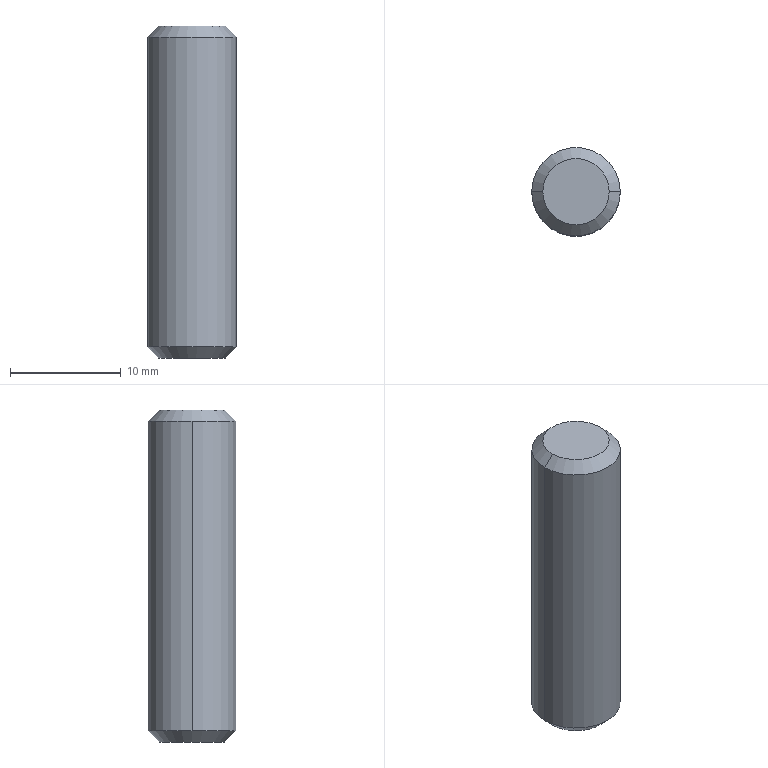Part | SolidWorks | features Chamfer 1, Extrusion 1 | 1 solid | 8 faces | box 8 x 8 x 30 mm | volume 1485 mm3 | cone 4 | cylinder 2 | plane 2 | commonest cylinder face diameters 8 x2
STEP:
#1=CARTESIAN_POINT('',(3.,0.,30.));
#2=VERTEX_POINT('',#1);
#3=CARTESIAN_POINT('',(-3.,0.,30.));
#4=VERTEX_POINT('',#3);
#5=CARTESIAN_POINT('',(0.,0.,30.));
#6=DIRECTION('',(0.,0.,1.));
#7=DIRECTION('',(1.,0.,0.));
#8=AXIS2_PLACEMENT_3D('',#5,#6,#7);
#9=CIRCLE('',#8,3.);
#10=EDGE_CURVE('',#2,#4,#9,.T.);
#11=ORIENTED_EDGE('',*,*,#10,.F.);
#12=CARTESIAN_POINT('',(4.,0.,29.));
#13=VERTEX_POINT('',#12);
#14=CARTESIAN_POINT('',(3.,0.,30.));
#15=DIRECTION('',(0.7071,0.,-0.7071));
#16=VECTOR('',#15,1000.);
#17=LINE('',#14,#16);
#18=EDGE_CURVE('',#2,#13,#17,.T.);
#19=ORIENTED_EDGE('',*,*,#18,.T.);
#20=CARTESIAN_POINT('',(-4.,0.,29.));
#21=VERTEX_POINT('',#20);
#22=CARTESIAN_POINT('',(0.,0.,29.));
#23=DIRECTION('',(0.,0.,-1.));
#24=DIRECTION('',(1.,0.,0.));
#25=AXIS2_PLACEMENT_3D('',#22,#23,#24);
#26=CIRCLE('',#25,4.);
#27=EDGE_CURVE('',#21,#13,#26,.T.);
#28=ORIENTED_EDGE('',*,*,#27,.F.);
#29=CARTESIAN_POINT('',(-3.,0.,30.));
#30=DIRECTION('',(-0.7071,0.,-0.7071));
#31=VECTOR('',#30,1000.);
#32=LINE('',#29,#31);
#33=EDGE_CURVE('',#4,#21,#32,.T.);
#34=ORIENTED_EDGE('',*,*,#33,.F.);
#35=EDGE_LOOP('',(#11,#19,#28,#34));
#36=FACE_OUTER_BOUND('',#35,.T.);
#37=CARTESIAN_POINT('',(0.,0.,30.));
#38=DIRECTION('',(0.,0.,-1.));
#39=DIRECTION('',(-1.,0.,0.));
#40=AXIS2_PLACEMENT_3D('',#37,#38,#39);
#41=CONICAL_SURFACE('',#40,3.,0.7854);
#42=ADVANCED_FACE('',(#36),#41,.T.);
#43=CARTESIAN_POINT('',(-3.,0.,0.));
#44=VERTEX_POINT('',#43);
#45=CARTESIAN_POINT('',(3.,0.,0.));
#46=VERTEX_POINT('',#45);
#47=CARTESIAN_POINT('',(0.,0.,0.));
#48=DIRECTION('',(0.,0.,-1.));
#49=DIRECTION('',(1.,0.,0.));
#50=AXIS2_PLACEMENT_3D('',#47,#48,#49);
#51=CIRCLE('',#50,3.);
#52=EDGE_CURVE('',#44,#46,#51,.T.);
#53=ORIENTED_EDGE('',*,*,#52,.F.);
#54=CARTESIAN_POINT('',(-4.,0.,1.));
#55=VERTEX_POINT('',#54);
#56=CARTESIAN_POINT('',(-4.,0.,1.));
#57=DIRECTION('',(-0.7071,0.,0.7071));
#58=VECTOR('',#57,1000.);
#59=LINE('',#56,#58);
#60=EDGE_CURVE('',#44,#55,#59,.T.);
#61=ORIENTED_EDGE('',*,*,#60,.T.);
#62=CARTESIAN_POINT('',(4.,0.,1.));
#63=VERTEX_POINT('',#62);
#64=CARTESIAN_POINT('',(0.,0.,1.));
#65=DIRECTION('',(0.,0.,1.));
#66=DIRECTION('',(1.,0.,0.));
#67=AXIS2_PLACEMENT_3D('',#64,#65,#66);
#68=CIRCLE('',#67,4.);
#69=EDGE_CURVE('',#63,#55,#68,.T.);
#70=ORIENTED_EDGE('',*,*,#69,.F.);
#71=CARTESIAN_POINT('',(4.,0.,1.));
#72=DIRECTION('',(0.7071,0.,0.7071));
#73=VECTOR('',#72,1000.);
#74=LINE('',#71,#73);
#75=EDGE_CURVE('',#46,#63,#74,.T.);
#76=ORIENTED_EDGE('',*,*,#75,.F.);
#77=EDGE_LOOP('',(#53,#61,#70,#76));
#78=FACE_OUTER_BOUND('',#77,.T.);
#79=CARTESIAN_POINT('',(0.,0.,1.));
#80=DIRECTION('',(0.,0.,1.));
#81=DIRECTION('',(1.,0.,0.));
#82=AXIS2_PLACEMENT_3D('',#79,#80,#81);
#83=CONICAL_SURFACE('',#82,4.,0.7854);
#84=ADVANCED_FACE('',(#78),#83,.T.);
#85=ORIENTED_EDGE('',*,*,#27,.T.);
#86=CARTESIAN_POINT('',(4.,0.,30.));
#87=DIRECTION('',(0.,0.,-1.));
#88=VECTOR('',#87,1000.);
#89=LINE('',#86,#88);
#90=EDGE_CURVE('',#13,#63,#89,.T.);
#91=ORIENTED_EDGE('',*,*,#90,.T.);
#92=ORIENTED_EDGE('',*,*,#69,.T.);
#93=CARTESIAN_POINT('',(-4.,0.,30.));
#94=DIRECTION('',(0.,0.,-1.));
#95=VECTOR('',#94,1000.);
#96=LINE('',#93,#95);
#97=EDGE_CURVE('',#21,#55,#96,.T.);
#98=ORIENTED_EDGE('',*,*,#97,.F.);
#99=EDGE_LOOP('',(#85,#91,#92,#98));
#100=FACE_OUTER_BOUND('',#99,.T.);
#101=CARTESIAN_POINT('',(0.,0.,30.));
#102=DIRECTION('',(0.,0.,-1.));
#103=DIRECTION('',(-1.,0.,0.));
#104=AXIS2_PLACEMENT_3D('',#101,#102,#103);
#105=CYLINDRICAL_SURFACE('',#104,4.);
#106=ADVANCED_FACE('',(#100),#105,.T.);
#107=ORIENTED_EDGE('',*,*,#90,.F.);
#108=CARTESIAN_POINT('',(0.,0.,29.));
#109=DIRECTION('',(0.,0.,-1.));
#110=DIRECTION('',(1.,0.,0.));
#111=AXIS2_PLACEMENT_3D('',#108,#109,#110);
#112=CIRCLE('',#111,4.);
#113=EDGE_CURVE('',#13,#21,#112,.T.);
#114=ORIENTED_EDGE('',*,*,#113,.T.);
#115=ORIENTED_EDGE('',*,*,#97,.T.);
#116=CARTESIAN_POINT('',(0.,0.,1.));
#117=DIRECTION('',(0.,0.,1.));
#118=DIRECTION('',(1.,0.,0.));
#119=AXIS2_PLACEMENT_3D('',#116,#117,#118);
#120=CIRCLE('',#119,4.);
#121=EDGE_CURVE('',#55,#63,#120,.T.);
#122=ORIENTED_EDGE('',*,*,#121,.T.);
#123=EDGE_LOOP('',(#107,#114,#115,#122));
#124=FACE_OUTER_BOUND('',#123,.T.);
#125=CARTESIAN_POINT('',(0.,0.,30.));
#126=DIRECTION('',(0.,0.,-1.));
#127=DIRECTION('',(-1.,0.,0.));
#128=AXIS2_PLACEMENT_3D('',#125,#126,#127);
#129=CYLINDRICAL_SURFACE('',#128,4.);
#130=ADVANCED_FACE('',(#124),#129,.T.);
#131=CARTESIAN_POINT('',(0.,0.,30.));
#132=DIRECTION('',(0.,0.,1.));
#133=DIRECTION('',(1.,0.,0.));
#134=AXIS2_PLACEMENT_3D('',#131,#132,#133);
#135=CIRCLE('',#134,3.);
#136=EDGE_CURVE('',#4,#2,#135,.T.);
#137=ORIENTED_EDGE('',*,*,#136,.T.);
#138=ORIENTED_EDGE('',*,*,#10,.T.);
#139=EDGE_LOOP('',(#137,#138));
#140=FACE_OUTER_BOUND('',#139,.T.);
#141=CARTESIAN_POINT('',(0.,0.,30.));
#142=DIRECTION('',(0.,0.,1.));
#143=DIRECTION('',(1.,0.,0.));
#144=AXIS2_PLACEMENT_3D('',#141,#142,#143);
#145=PLANE('',#144);
#146=ADVANCED_FACE('',(#140),#145,.T.);
#147=CARTESIAN_POINT('',(0.,0.,0.));
#148=DIRECTION('',(0.,0.,-1.));
#149=DIRECTION('',(1.,0.,0.));
#150=AXIS2_PLACEMENT_3D('',#147,#148,#149);
#151=CIRCLE('',#150,3.);
#152=EDGE_CURVE('',#46,#44,#151,.T.);
#153=ORIENTED_EDGE('',*,*,#152,.T.);
#154=ORIENTED_EDGE('',*,*,#52,.T.);
#155=EDGE_LOOP('',(#153,#154));
#156=FACE_OUTER_BOUND('',#155,.T.);
#157=CARTESIAN_POINT('',(0.,0.,0.));
#158=DIRECTION('',(0.,0.,1.));
#159=DIRECTION('',(1.,0.,0.));
#160=AXIS2_PLACEMENT_3D('',#157,#158,#159);
#161=PLANE('',#160);
#162=ADVANCED_FACE('',(#156),#161,.F.);
#163=ORIENTED_EDGE('',*,*,#60,.F.);
#164=ORIENTED_EDGE('',*,*,#152,.F.);
#165=ORIENTED_EDGE('',*,*,#75,.T.);
#166=ORIENTED_EDGE('',*,*,#121,.F.);
#167=EDGE_LOOP('',(#163,#164,#165,#166));
#168=FACE_OUTER_BOUND('',#167,.T.);
#169=CARTESIAN_POINT('',(0.,0.,1.));
#170=DIRECTION('',(0.,0.,1.));
#171=DIRECTION('',(1.,0.,0.));
#172=AXIS2_PLACEMENT_3D('',#169,#170,#171);
#173=CONICAL_SURFACE('',#172,4.,0.7854);
#174=ADVANCED_FACE('',(#168),#173,.T.);
#175=ORIENTED_EDGE('',*,*,#18,.F.);
#176=ORIENTED_EDGE('',*,*,#136,.F.);
#177=ORIENTED_EDGE('',*,*,#33,.T.);
#178=ORIENTED_EDGE('',*,*,#113,.F.);
#179=EDGE_LOOP('',(#175,#176,#177,#178));
#180=FACE_OUTER_BOUND('',#179,.T.);
#181=CARTESIAN_POINT('',(0.,0.,30.));
#182=DIRECTION('',(0.,0.,-1.));
#183=DIRECTION('',(-1.,0.,0.));
#184=AXIS2_PLACEMENT_3D('',#181,#182,#183);
#185=CONICAL_SURFACE('',#184,3.,0.7854);
#186=ADVANCED_FACE('',(#180),#185,.T.);
#187=CLOSED_SHELL('',(#42,#84,#106,#130,#146,#162,#174,#186));
#188=MANIFOLD_SOLID_BREP('',#187);
#189=CARTESIAN_POINT('',(0.,0.,0.));
#190=DIRECTION('',(0.,0.,1.));
#191=DIRECTION('',(1.,0.,0.));
#192=AXIS2_PLACEMENT_3D('',#189,#190,#191);
#193=(LENGTH_UNIT()NAMED_UNIT(*)SI_UNIT(.MILLI.,.METRE.));
#194=UNCERTAINTY_MEASURE_WITH_UNIT(LENGTH_MEASURE(0.00001),#193,'','');
#195=(NAMED_UNIT(*)PLANE_ANGLE_UNIT()SI_UNIT($,.RADIAN.));
#196=(NAMED_UNIT(*)SI_UNIT($,.STERADIAN.)SOLID_ANGLE_UNIT());
#197=(GEOMETRIC_REPRESENTATION_CONTEXT(3)GLOBAL_UNCERTAINTY_ASSIGNED_CONTEXT((#194))GLOBAL_UNIT_ASSIGNED_CONTEXT((#193,#195,#196))REPRESENTATION_CONTEXT('',''));
#198=ADVANCED_BREP_SHAPE_REPRESENTATION('',(#188,#192),#197);